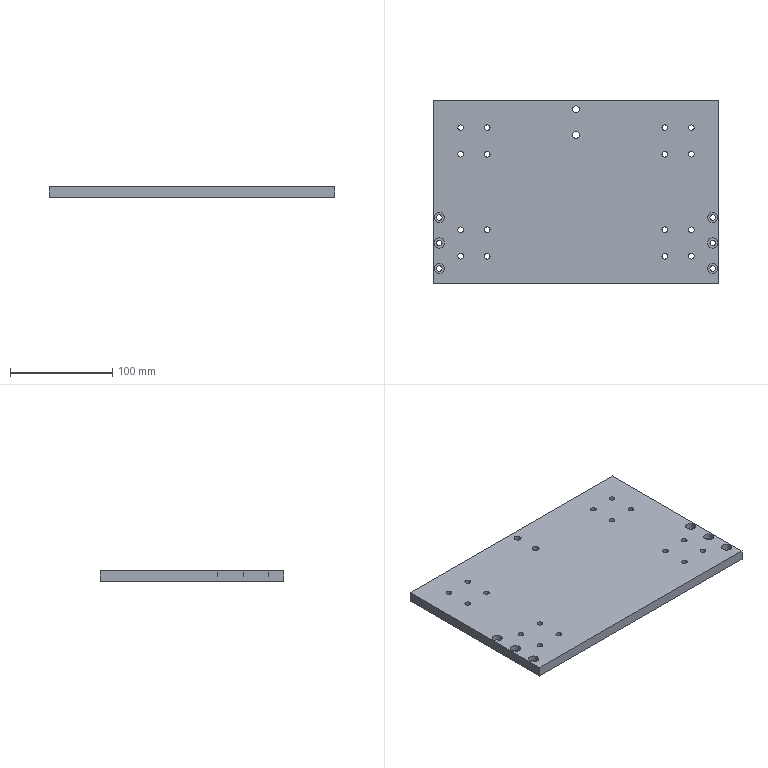Part | STEP file | PN_0028 (connecting block) | 1 solid | 120 faces | box 280 x 180 x 10 mm | volume 491440 mm3 | cylinder 92 | plane 28 | commonest cylinder face diameters 5.5 x44 10 x44 6.8 x4